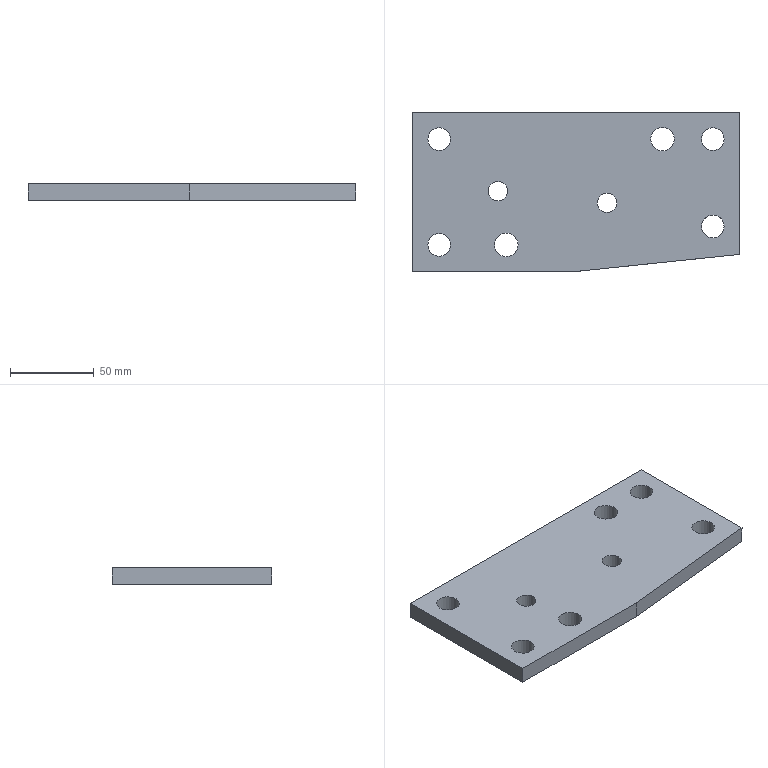Part | STEP file | lll_id2958_x_t | 1 solid | 15 faces | box 195 x 95 x 10 mm | volume 169241 mm3 | cylinder 8 | plane 7 | commonest cylinder face diameters 13.509 x4 11.508 x2 14 x2
STEP:
#1=CARTESIAN_POINT('',(329.746,24.75,92.5));
#2=VERTEX_POINT('',#1);
#3=CARTESIAN_POINT('',(335.5,24.75,92.5));
#4=DIRECTION('',(0.,0.,1.));
#5=DIRECTION('',(-1.,0.,0.));
#6=AXIS2_PLACEMENT_3D('',#3,#4,#5);
#7=CIRCLE('',#6,5.754);
#8=EDGE_CURVE('',#2,#2,#7,.T.);
#9=ORIENTED_EDGE('',*,*,#8,.T.);
#10=EDGE_LOOP('',(#9));
#11=FACE_BOUND('',#10,.T.);
#12=CARTESIAN_POINT('',(380.426,-23.25,92.5));
#13=VERTEX_POINT('',#12);
#14=CARTESIAN_POINT('',(479.5,-12.921,92.5));
#15=VERTEX_POINT('',#14);
#16=CARTESIAN_POINT('',(386.882,-22.577,92.5));
#17=DIRECTION('',(0.9946,0.1037,0.));
#18=VECTOR('',#17,1.);
#19=LINE('',#16,#18);
#20=EDGE_CURVE('',#13,#15,#19,.T.);
#21=ORIENTED_EDGE('',*,*,#20,.F.);
#22=CARTESIAN_POINT('',(284.5,-23.25,92.5));
#23=VERTEX_POINT('',#22);
#24=CARTESIAN_POINT('',(382.,-23.25,92.5));
#25=DIRECTION('',(1.,0.,0.));
#26=VECTOR('',#25,1.);
#27=LINE('',#24,#26);
#28=EDGE_CURVE('',#23,#13,#27,.T.);
#29=ORIENTED_EDGE('',*,*,#28,.F.);
#30=CARTESIAN_POINT('',(284.5,71.75,92.5));
#31=VERTEX_POINT('',#30);
#32=CARTESIAN_POINT('',(284.5,24.25,92.5));
#33=DIRECTION('',(0.,-1.,0.));
#34=VECTOR('',#33,1.);
#35=LINE('',#32,#34);
#36=EDGE_CURVE('',#31,#23,#35,.T.);
#37=ORIENTED_EDGE('',*,*,#36,.F.);
#38=CARTESIAN_POINT('',(479.5,71.75,92.5));
#39=VERTEX_POINT('',#38);
#40=CARTESIAN_POINT('',(382.,71.75,92.5));
#41=DIRECTION('',(-1.,0.,0.));
#42=VECTOR('',#41,1.);
#43=LINE('',#40,#42);
#44=EDGE_CURVE('',#39,#31,#43,.T.);
#45=ORIENTED_EDGE('',*,*,#44,.F.);
#46=CARTESIAN_POINT('',(479.5,24.25,92.5));
#47=DIRECTION('',(0.,1.,0.));
#48=VECTOR('',#47,1.);
#49=LINE('',#46,#48);
#50=EDGE_CURVE('',#15,#39,#49,.T.);
#51=ORIENTED_EDGE('',*,*,#50,.F.);
#52=EDGE_LOOP('',(#21,#29,#37,#45,#51));
#53=FACE_BOUND('',#52,.T.);
#54=CARTESIAN_POINT('',(426.5,55.75,92.5));
#55=VERTEX_POINT('',#54);
#56=CARTESIAN_POINT('',(433.5,55.75,92.5));
#57=DIRECTION('',(0.,0.,1.));
#58=DIRECTION('',(-1.,0.,0.));
#59=AXIS2_PLACEMENT_3D('',#56,#57,#58);
#60=CIRCLE('',#59,7.);
#61=EDGE_CURVE('',#55,#55,#60,.T.);
#62=ORIENTED_EDGE('',*,*,#61,.T.);
#63=EDGE_LOOP('',(#62));
#64=FACE_BOUND('',#63,.T.);
#65=CARTESIAN_POINT('',(293.745,55.75,92.5));
#66=VERTEX_POINT('',#65);
#67=CARTESIAN_POINT('',(300.5,55.75,92.5));
#68=DIRECTION('',(0.,0.,1.));
#69=DIRECTION('',(-1.,0.,0.));
#70=AXIS2_PLACEMENT_3D('',#67,#68,#69);
#71=CIRCLE('',#70,6.755);
#72=EDGE_CURVE('',#66,#66,#71,.T.);
#73=ORIENTED_EDGE('',*,*,#72,.T.);
#74=EDGE_LOOP('',(#73));
#75=FACE_BOUND('',#74,.T.);
#76=CARTESIAN_POINT('',(456.745,55.75,92.5));
#77=VERTEX_POINT('',#76);
#78=CARTESIAN_POINT('',(463.5,55.75,92.5));
#79=DIRECTION('',(0.,0.,1.));
#80=DIRECTION('',(-1.,0.,0.));
#81=AXIS2_PLACEMENT_3D('',#78,#79,#80);
#82=CIRCLE('',#81,6.755);
#83=EDGE_CURVE('',#77,#77,#82,.T.);
#84=ORIENTED_EDGE('',*,*,#83,.T.);
#85=EDGE_LOOP('',(#84));
#86=FACE_BOUND('',#85,.T.);
#87=CARTESIAN_POINT('',(293.745,-7.25,92.5));
#88=VERTEX_POINT('',#87);
#89=CARTESIAN_POINT('',(300.5,-7.25,92.5));
#90=DIRECTION('',(0.,0.,1.));
#91=DIRECTION('',(-1.,0.,0.));
#92=AXIS2_PLACEMENT_3D('',#89,#90,#91);
#93=CIRCLE('',#92,6.755);
#94=EDGE_CURVE('',#88,#88,#93,.T.);
#95=ORIENTED_EDGE('',*,*,#94,.T.);
#96=EDGE_LOOP('',(#95));
#97=FACE_BOUND('',#96,.T.);
#98=CARTESIAN_POINT('',(456.745,3.75,92.5));
#99=VERTEX_POINT('',#98);
#100=CARTESIAN_POINT('',(463.5,3.75,92.5));
#101=DIRECTION('',(0.,0.,1.));
#102=DIRECTION('',(-1.,0.,0.));
#103=AXIS2_PLACEMENT_3D('',#100,#101,#102);
#104=CIRCLE('',#103,6.755);
#105=EDGE_CURVE('',#99,#99,#104,.T.);
#106=ORIENTED_EDGE('',*,*,#105,.T.);
#107=EDGE_LOOP('',(#106));
#108=FACE_BOUND('',#107,.T.);
#109=CARTESIAN_POINT('',(333.5,-7.25,92.5));
#110=VERTEX_POINT('',#109);
#111=CARTESIAN_POINT('',(340.5,-7.25,92.5));
#112=DIRECTION('',(0.,0.,1.));
#113=DIRECTION('',(-1.,0.,0.));
#114=AXIS2_PLACEMENT_3D('',#111,#112,#113);
#115=CIRCLE('',#114,7.);
#116=EDGE_CURVE('',#110,#110,#115,.T.);
#117=ORIENTED_EDGE('',*,*,#116,.T.);
#118=EDGE_LOOP('',(#117));
#119=FACE_BOUND('',#118,.T.);
#120=CARTESIAN_POINT('',(394.746,17.75,92.5));
#121=VERTEX_POINT('',#120);
#122=CARTESIAN_POINT('',(400.5,17.75,92.5));
#123=DIRECTION('',(0.,0.,1.));
#124=DIRECTION('',(-1.,0.,0.));
#125=AXIS2_PLACEMENT_3D('',#122,#123,#124);
#126=CIRCLE('',#125,5.754);
#127=EDGE_CURVE('',#121,#121,#126,.T.);
#128=ORIENTED_EDGE('',*,*,#127,.T.);
#129=EDGE_LOOP('',(#128));
#130=FACE_BOUND('',#129,.T.);
#131=CARTESIAN_POINT('',(382.,24.25,92.5));
#132=DIRECTION('',(0.,0.,-1.));
#133=DIRECTION('',(1.,0.,0.));
#134=AXIS2_PLACEMENT_3D('',#131,#132,#133);
#135=PLANE('',#134);
#136=ADVANCED_FACE('',(#11,#53,#64,#75,#86,#97,#108,#119,#130),#135,.T.);
#137=CARTESIAN_POINT('',(479.5,71.75,102.5));
#138=VERTEX_POINT('',#137);
#139=CARTESIAN_POINT('',(284.5,71.75,102.5));
#140=VERTEX_POINT('',#139);
#141=CARTESIAN_POINT('',(382.,71.75,102.5));
#142=DIRECTION('',(-1.,0.,0.));
#143=VECTOR('',#142,1.);
#144=LINE('',#141,#143);
#145=EDGE_CURVE('',#138,#140,#144,.T.);
#146=ORIENTED_EDGE('',*,*,#145,.F.);
#147=CARTESIAN_POINT('',(479.5,71.75,92.5));
#148=DIRECTION('',(0.,0.,1.));
#149=VECTOR('',#148,1.);
#150=LINE('',#147,#149);
#151=EDGE_CURVE('',#39,#138,#150,.T.);
#152=ORIENTED_EDGE('',*,*,#151,.F.);
#153=ORIENTED_EDGE('',*,*,#44,.T.);
#154=CARTESIAN_POINT('',(284.5,71.75,92.5));
#155=DIRECTION('',(0.,0.,1.));
#156=VECTOR('',#155,1.);
#157=LINE('',#154,#156);
#158=EDGE_CURVE('',#31,#140,#157,.T.);
#159=ORIENTED_EDGE('',*,*,#158,.T.);
#160=EDGE_LOOP('',(#146,#152,#153,#159));
#161=FACE_OUTER_BOUND('',#160,.T.);
#162=CARTESIAN_POINT('',(382.,71.75,92.5));
#163=DIRECTION('',(0.,1.,0.));
#164=DIRECTION('',(0.,0.,-1.));
#165=AXIS2_PLACEMENT_3D('',#162,#163,#164);
#166=PLANE('',#165);
#167=ADVANCED_FACE('',(#161),#166,.T.);
#168=CARTESIAN_POINT('',(479.5,-12.921,102.5));
#169=VERTEX_POINT('',#168);
#170=CARTESIAN_POINT('',(479.5,24.25,102.5));
#171=DIRECTION('',(0.,-1.,0.));
#172=VECTOR('',#171,1.);
#173=LINE('',#170,#172);
#174=EDGE_CURVE('',#138,#169,#173,.T.);
#175=ORIENTED_EDGE('',*,*,#174,.T.);
#176=CARTESIAN_POINT('',(479.5,-12.921,92.5));
#177=DIRECTION('',(0.,0.,1.));
#178=VECTOR('',#177,1.);
#179=LINE('',#176,#178);
#180=EDGE_CURVE('',#15,#169,#179,.T.);
#181=ORIENTED_EDGE('',*,*,#180,.F.);
#182=ORIENTED_EDGE('',*,*,#50,.T.);
#183=ORIENTED_EDGE('',*,*,#151,.T.);
#184=EDGE_LOOP('',(#175,#181,#182,#183));
#185=FACE_OUTER_BOUND('',#184,.T.);
#186=CARTESIAN_POINT('',(479.5,24.25,92.5));
#187=DIRECTION('',(1.,0.,0.));
#188=DIRECTION('',(0.,0.,1.));
#189=AXIS2_PLACEMENT_3D('',#186,#187,#188);
#190=PLANE('',#189);
#191=ADVANCED_FACE('',(#185),#190,.T.);
#192=CARTESIAN_POINT('',(284.5,-23.25,102.5));
#193=VERTEX_POINT('',#192);
#194=CARTESIAN_POINT('',(380.426,-23.25,102.5));
#195=VERTEX_POINT('',#194);
#196=CARTESIAN_POINT('',(382.,-23.25,102.5));
#197=DIRECTION('',(1.,0.,0.));
#198=VECTOR('',#197,1.);
#199=LINE('',#196,#198);
#200=EDGE_CURVE('',#193,#195,#199,.T.);
#201=ORIENTED_EDGE('',*,*,#200,.F.);
#202=CARTESIAN_POINT('',(284.5,-23.25,92.5));
#203=DIRECTION('',(0.,0.,1.));
#204=VECTOR('',#203,1.);
#205=LINE('',#202,#204);
#206=EDGE_CURVE('',#23,#193,#205,.T.);
#207=ORIENTED_EDGE('',*,*,#206,.F.);
#208=ORIENTED_EDGE('',*,*,#28,.T.);
#209=CARTESIAN_POINT('',(380.426,-23.25,92.5));
#210=DIRECTION('',(0.,0.,-1.));
#211=VECTOR('',#210,1.);
#212=LINE('',#209,#211);
#213=EDGE_CURVE('',#195,#13,#212,.T.);
#214=ORIENTED_EDGE('',*,*,#213,.F.);
#215=EDGE_LOOP('',(#201,#207,#208,#214));
#216=FACE_OUTER_BOUND('',#215,.T.);
#217=CARTESIAN_POINT('',(382.,-23.25,92.5));
#218=DIRECTION('',(0.,-1.,0.));
#219=DIRECTION('',(0.,0.,1.));
#220=AXIS2_PLACEMENT_3D('',#217,#218,#219);
#221=PLANE('',#220);
#222=ADVANCED_FACE('',(#216),#221,.T.);
#223=CARTESIAN_POINT('',(284.5,24.25,102.5));
#224=DIRECTION('',(0.,1.,0.));
#225=VECTOR('',#224,1.);
#226=LINE('',#223,#225);
#227=EDGE_CURVE('',#193,#140,#226,.T.);
#228=ORIENTED_EDGE('',*,*,#227,.T.);
#229=ORIENTED_EDGE('',*,*,#158,.F.);
#230=ORIENTED_EDGE('',*,*,#36,.T.);
#231=ORIENTED_EDGE('',*,*,#206,.T.);
#232=EDGE_LOOP('',(#228,#229,#230,#231));
#233=FACE_OUTER_BOUND('',#232,.T.);
#234=CARTESIAN_POINT('',(284.5,24.25,92.5));
#235=DIRECTION('',(-1.,0.,0.));
#236=DIRECTION('',(0.,0.,-1.));
#237=AXIS2_PLACEMENT_3D('',#234,#235,#236);
#238=PLANE('',#237);
#239=ADVANCED_FACE('',(#233),#238,.T.);
#240=CARTESIAN_POINT('',(456.745,55.75,102.5));
#241=VERTEX_POINT('',#240);
#242=CARTESIAN_POINT('',(463.5,55.75,102.5));
#243=DIRECTION('',(0.,0.,-1.));
#244=DIRECTION('',(-1.,0.,0.));
#245=AXIS2_PLACEMENT_3D('',#242,#243,#244);
#246=CIRCLE('',#245,6.755);
#247=EDGE_CURVE('',#241,#241,#246,.T.);
#248=ORIENTED_EDGE('',*,*,#247,.F.);
#249=EDGE_LOOP('',(#248));
#250=FACE_BOUND('',#249,.T.);
#251=ORIENTED_EDGE('',*,*,#83,.F.);
#252=EDGE_LOOP('',(#251));
#253=FACE_BOUND('',#252,.T.);
#254=CARTESIAN_POINT('',(463.5,55.75,92.5));
#255=DIRECTION('',(0.,0.,1.));
#256=DIRECTION('',(-1.,0.,0.));
#257=AXIS2_PLACEMENT_3D('',#254,#255,#256);
#258=CYLINDRICAL_SURFACE('',#257,6.755);
#259=ADVANCED_FACE('',(#250,#253),#258,.F.);
#260=CARTESIAN_POINT('',(293.745,-7.25,102.5));
#261=VERTEX_POINT('',#260);
#262=CARTESIAN_POINT('',(300.5,-7.25,102.5));
#263=DIRECTION('',(0.,0.,-1.));
#264=DIRECTION('',(-1.,0.,0.));
#265=AXIS2_PLACEMENT_3D('',#262,#263,#264);
#266=CIRCLE('',#265,6.755);
#267=EDGE_CURVE('',#261,#261,#266,.T.);
#268=ORIENTED_EDGE('',*,*,#267,.F.);
#269=EDGE_LOOP('',(#268));
#270=FACE_BOUND('',#269,.T.);
#271=ORIENTED_EDGE('',*,*,#94,.F.);
#272=EDGE_LOOP('',(#271));
#273=FACE_BOUND('',#272,.T.);
#274=CARTESIAN_POINT('',(300.5,-7.25,92.5));
#275=DIRECTION('',(0.,0.,1.));
#276=DIRECTION('',(-1.,0.,0.));
#277=AXIS2_PLACEMENT_3D('',#274,#275,#276);
#278=CYLINDRICAL_SURFACE('',#277,6.755);
#279=ADVANCED_FACE('',(#270,#273),#278,.F.);
#280=CARTESIAN_POINT('',(293.745,55.75,102.5));
#281=VERTEX_POINT('',#280);
#282=CARTESIAN_POINT('',(300.5,55.75,102.5));
#283=DIRECTION('',(0.,0.,1.));
#284=DIRECTION('',(-1.,0.,0.));
#285=AXIS2_PLACEMENT_3D('',#282,#283,#284);
#286=CIRCLE('',#285,6.755);
#287=EDGE_CURVE('',#281,#281,#286,.T.);
#288=ORIENTED_EDGE('',*,*,#287,.T.);
#289=EDGE_LOOP('',(#288));
#290=FACE_BOUND('',#289,.T.);
#291=ORIENTED_EDGE('',*,*,#72,.F.);
#292=EDGE_LOOP('',(#291));
#293=FACE_BOUND('',#292,.T.);
#294=CARTESIAN_POINT('',(300.5,55.75,92.5));
#295=DIRECTION('',(0.,0.,1.));
#296=DIRECTION('',(-1.,0.,0.));
#297=AXIS2_PLACEMENT_3D('',#294,#295,#296);
#298=CYLINDRICAL_SURFACE('',#297,6.755);
#299=ADVANCED_FACE('',(#290,#293),#298,.F.);
#300=CARTESIAN_POINT('',(456.745,3.75,102.5));
#301=VERTEX_POINT('',#300);
#302=CARTESIAN_POINT('',(463.5,3.75,102.5));
#303=DIRECTION('',(0.,0.,-1.));
#304=DIRECTION('',(-1.,0.,0.));
#305=AXIS2_PLACEMENT_3D('',#302,#303,#304);
#306=CIRCLE('',#305,6.755);
#307=EDGE_CURVE('',#301,#301,#306,.T.);
#308=ORIENTED_EDGE('',*,*,#307,.F.);
#309=EDGE_LOOP('',(#308));
#310=FACE_BOUND('',#309,.T.);
#311=ORIENTED_EDGE('',*,*,#105,.F.);
#312=EDGE_LOOP('',(#311));
#313=FACE_BOUND('',#312,.T.);
#314=CARTESIAN_POINT('',(463.5,3.75,92.5));
#315=DIRECTION('',(0.,0.,1.));
#316=DIRECTION('',(-1.,0.,0.));
#317=AXIS2_PLACEMENT_3D('',#314,#315,#316);
#318=CYLINDRICAL_SURFACE('',#317,6.755);
#319=ADVANCED_FACE('',(#310,#313),#318,.F.);
#320=CARTESIAN_POINT('',(426.5,55.75,102.5));
#321=VERTEX_POINT('',#320);
#322=CARTESIAN_POINT('',(433.5,55.75,102.5));
#323=DIRECTION('',(0.,0.,-1.));
#324=DIRECTION('',(-1.,0.,0.));
#325=AXIS2_PLACEMENT_3D('',#322,#323,#324);
#326=CIRCLE('',#325,7.);
#327=EDGE_CURVE('',#321,#321,#326,.T.);
#328=ORIENTED_EDGE('',*,*,#327,.F.);
#329=EDGE_LOOP('',(#328));
#330=FACE_BOUND('',#329,.T.);
#331=ORIENTED_EDGE('',*,*,#61,.F.);
#332=EDGE_LOOP('',(#331));
#333=FACE_BOUND('',#332,.T.);
#334=CARTESIAN_POINT('',(433.5,55.75,92.5));
#335=DIRECTION('',(0.,0.,1.));
#336=DIRECTION('',(-1.,0.,0.));
#337=AXIS2_PLACEMENT_3D('',#334,#335,#336);
#338=CYLINDRICAL_SURFACE('',#337,7.);
#339=ADVANCED_FACE('',(#330,#333),#338,.F.);
#340=CARTESIAN_POINT('',(333.5,-7.25,102.5));
#341=VERTEX_POINT('',#340);
#342=CARTESIAN_POINT('',(340.5,-7.25,102.5));
#343=DIRECTION('',(0.,0.,1.));
#344=DIRECTION('',(-1.,0.,0.));
#345=AXIS2_PLACEMENT_3D('',#342,#343,#344);
#346=CIRCLE('',#345,7.);
#347=EDGE_CURVE('',#341,#341,#346,.T.);
#348=ORIENTED_EDGE('',*,*,#347,.T.);
#349=EDGE_LOOP('',(#348));
#350=FACE_BOUND('',#349,.T.);
#351=ORIENTED_EDGE('',*,*,#116,.F.);
#352=EDGE_LOOP('',(#351));
#353=FACE_BOUND('',#352,.T.);
#354=CARTESIAN_POINT('',(340.5,-7.25,92.5));
#355=DIRECTION('',(0.,0.,1.));
#356=DIRECTION('',(-1.,0.,0.));
#357=AXIS2_PLACEMENT_3D('',#354,#355,#356);
#358=CYLINDRICAL_SURFACE('',#357,7.);
#359=ADVANCED_FACE('',(#350,#353),#358,.F.);
#360=ORIENTED_EDGE('',*,*,#180,.T.);
#361=CARTESIAN_POINT('',(479.344,-12.938,102.5));
#362=DIRECTION('',(-0.9946,-0.1037,0.));
#363=VECTOR('',#362,1.);
#364=LINE('',#361,#363);
#365=EDGE_CURVE('',#169,#195,#364,.T.);
#366=ORIENTED_EDGE('',*,*,#365,.T.);
#367=ORIENTED_EDGE('',*,*,#213,.T.);
#368=ORIENTED_EDGE('',*,*,#20,.T.);
#369=EDGE_LOOP('',(#360,#366,#367,#368));
#370=FACE_OUTER_BOUND('',#369,.T.);
#371=CARTESIAN_POINT('',(479.344,-12.938,-1360.5));
#372=DIRECTION('',(-0.1037,0.9946,0.));
#373=DIRECTION('',(-0.9946,-0.1037,0.));
#374=AXIS2_PLACEMENT_3D('',#371,#372,#373);
#375=PLANE('',#374);
#376=ADVANCED_FACE('',(#370),#375,.F.);
#377=CARTESIAN_POINT('',(329.746,24.75,102.5));
#378=VERTEX_POINT('',#377);
#379=CARTESIAN_POINT('',(335.5,24.75,102.5));
#380=DIRECTION('',(0.,0.,1.));
#381=DIRECTION('',(-1.,0.,0.));
#382=AXIS2_PLACEMENT_3D('',#379,#380,#381);
#383=CIRCLE('',#382,5.754);
#384=EDGE_CURVE('',#378,#378,#383,.T.);
#385=ORIENTED_EDGE('',*,*,#384,.T.);
#386=EDGE_LOOP('',(#385));
#387=FACE_BOUND('',#386,.T.);
#388=ORIENTED_EDGE('',*,*,#8,.F.);
#389=EDGE_LOOP('',(#388));
#390=FACE_BOUND('',#389,.T.);
#391=CARTESIAN_POINT('',(335.5,24.75,217.5));
#392=DIRECTION('',(0.,0.,-1.));
#393=DIRECTION('',(-1.,0.,0.));
#394=AXIS2_PLACEMENT_3D('',#391,#392,#393);
#395=CYLINDRICAL_SURFACE('',#394,5.754);
#396=ADVANCED_FACE('',(#387,#390),#395,.F.);
#397=CARTESIAN_POINT('',(394.746,17.75,102.5));
#398=VERTEX_POINT('',#397);
#399=CARTESIAN_POINT('',(400.5,17.75,102.5));
#400=DIRECTION('',(0.,0.,-1.));
#401=DIRECTION('',(-1.,0.,0.));
#402=AXIS2_PLACEMENT_3D('',#399,#400,#401);
#403=CIRCLE('',#402,5.754);
#404=EDGE_CURVE('',#398,#398,#403,.T.);
#405=ORIENTED_EDGE('',*,*,#404,.F.);
#406=EDGE_LOOP('',(#405));
#407=FACE_BOUND('',#406,.T.);
#408=ORIENTED_EDGE('',*,*,#127,.F.);
#409=EDGE_LOOP('',(#408));
#410=FACE_BOUND('',#409,.T.);
#411=CARTESIAN_POINT('',(400.5,17.75,217.5));
#412=DIRECTION('',(0.,0.,-1.));
#413=DIRECTION('',(-1.,0.,0.));
#414=AXIS2_PLACEMENT_3D('',#411,#412,#413);
#415=CYLINDRICAL_SURFACE('',#414,5.754);
#416=ADVANCED_FACE('',(#407,#410),#415,.F.);
#417=ORIENTED_EDGE('',*,*,#267,.T.);
#418=EDGE_LOOP('',(#417));
#419=FACE_BOUND('',#418,.T.);
#420=ORIENTED_EDGE('',*,*,#307,.T.);
#421=EDGE_LOOP('',(#420));
#422=FACE_BOUND('',#421,.T.);
#423=ORIENTED_EDGE('',*,*,#347,.F.);
#424=EDGE_LOOP('',(#423));
#425=FACE_BOUND('',#424,.T.);
#426=ORIENTED_EDGE('',*,*,#227,.F.);
#427=ORIENTED_EDGE('',*,*,#200,.T.);
#428=ORIENTED_EDGE('',*,*,#365,.F.);
#429=ORIENTED_EDGE('',*,*,#174,.F.);
#430=ORIENTED_EDGE('',*,*,#145,.T.);
#431=EDGE_LOOP('',(#426,#427,#428,#429,#430));
#432=FACE_BOUND('',#431,.T.);
#433=ORIENTED_EDGE('',*,*,#384,.F.);
#434=EDGE_LOOP('',(#433));
#435=FACE_BOUND('',#434,.T.);
#436=ORIENTED_EDGE('',*,*,#404,.T.);
#437=EDGE_LOOP('',(#436));
#438=FACE_BOUND('',#437,.T.);
#439=ORIENTED_EDGE('',*,*,#327,.T.);
#440=EDGE_LOOP('',(#439));
#441=FACE_BOUND('',#440,.T.);
#442=ORIENTED_EDGE('',*,*,#287,.F.);
#443=EDGE_LOOP('',(#442));
#444=FACE_BOUND('',#443,.T.);
#445=ORIENTED_EDGE('',*,*,#247,.T.);
#446=EDGE_LOOP('',(#445));
#447=FACE_BOUND('',#446,.T.);
#448=CARTESIAN_POINT('',(741.5,-0.002299,102.5));
#449=DIRECTION('',(0.,0.,-1.));
#450=DIRECTION('',(-1.,0.,0.));
#451=AXIS2_PLACEMENT_3D('',#448,#449,#450);
#452=PLANE('',#451);
#453=ADVANCED_FACE('',(#419,#422,#425,#432,#435,#438,#441,#444,#447),#452,.F.);
#454=CLOSED_SHELL('',(#136,#167,#191,#222,#239,#259,#279,#299,#319,#339,#359,#376,#396,#416,#453));
#455=MANIFOLD_SOLID_BREP('',#454);
#456=(LENGTH_UNIT()NAMED_UNIT(*)SI_UNIT(.MILLI.,.METRE.));
#457=UNCERTAINTY_MEASURE_WITH_UNIT(LENGTH_MEASURE(0.00002),#456,'','');
#458=(NAMED_UNIT(*)PLANE_ANGLE_UNIT()SI_UNIT($,.RADIAN.));
#459=PLANE_ANGLE_MEASURE_WITH_UNIT(PLANE_ANGLE_MEASURE(0.01745),#458);
#460=DIMENSIONAL_EXPONENTS(0.,0.,0.,0.,0.,0.,0.);
#461=(CONVERSION_BASED_UNIT('DEGREE',#459)NAMED_UNIT(#460)PLANE_ANGLE_UNIT());
#462=(NAMED_UNIT(*)SI_UNIT($,.STERADIAN.)SOLID_ANGLE_UNIT());
#463=(GEOMETRIC_REPRESENTATION_CONTEXT(3)GLOBAL_UNCERTAINTY_ASSIGNED_CONTEXT((#457))GLOBAL_UNIT_ASSIGNED_CONTEXT((#456,#461,#462))REPRESENTATION_CONTEXT('',''));
#464=ADVANCED_BREP_SHAPE_REPRESENTATION('',(#455),#463);